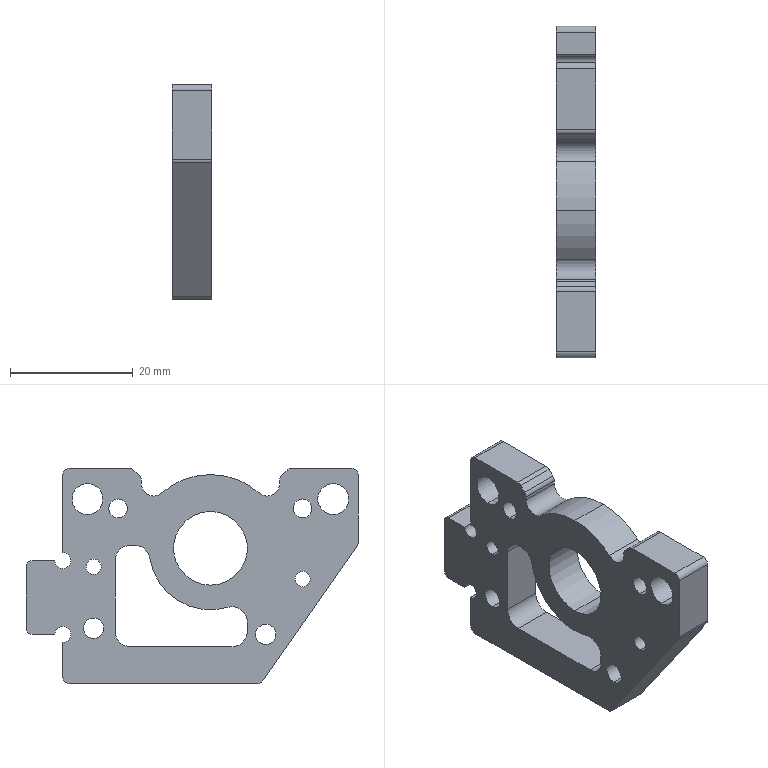Part | SolidWorks | features HoleWzd 3, Fillet 2, Chamfer 1, Extrusion 1 | 1 solid | 71 faces | box 6.5 x 54 x 35 mm | volume 7066 mm3 | cylinder 47 | plane 20 | cone 4 | commonest cylinder face diameters 2 x11 3.3 x8 5 x6 2.5 x4 3.05 x4 5.05 x4